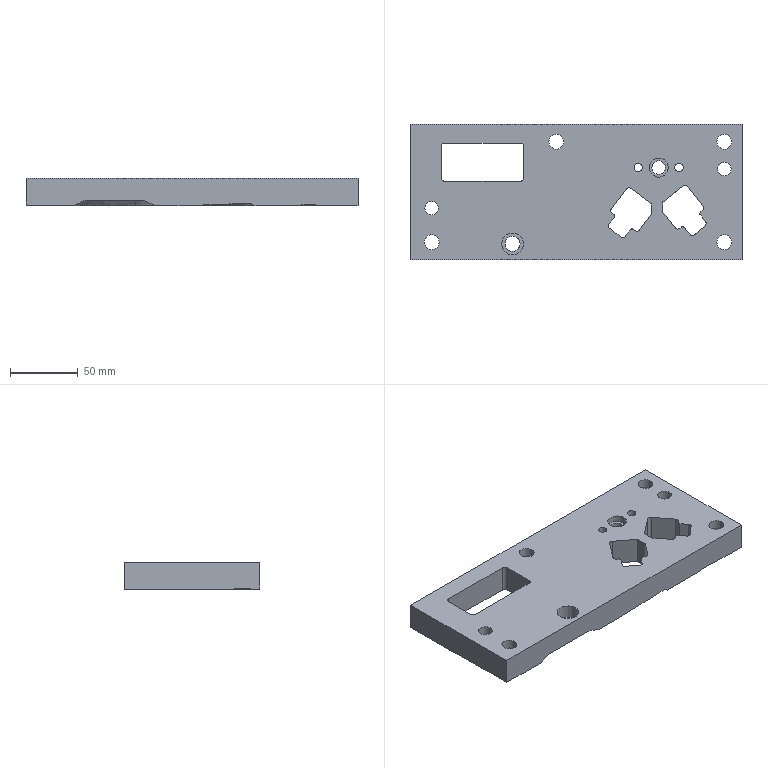Part | STEP file | 427_id1206_x_t | 1 solid | 112 faces | box 245 x 100 x 20.194 mm | volume 395706 mm3 | plane 38 | spline 38 | cylinder 36 | commonest cylinder face diameters 5 x10 11 x6 3 x4 4 x4 17 x4 10 x3